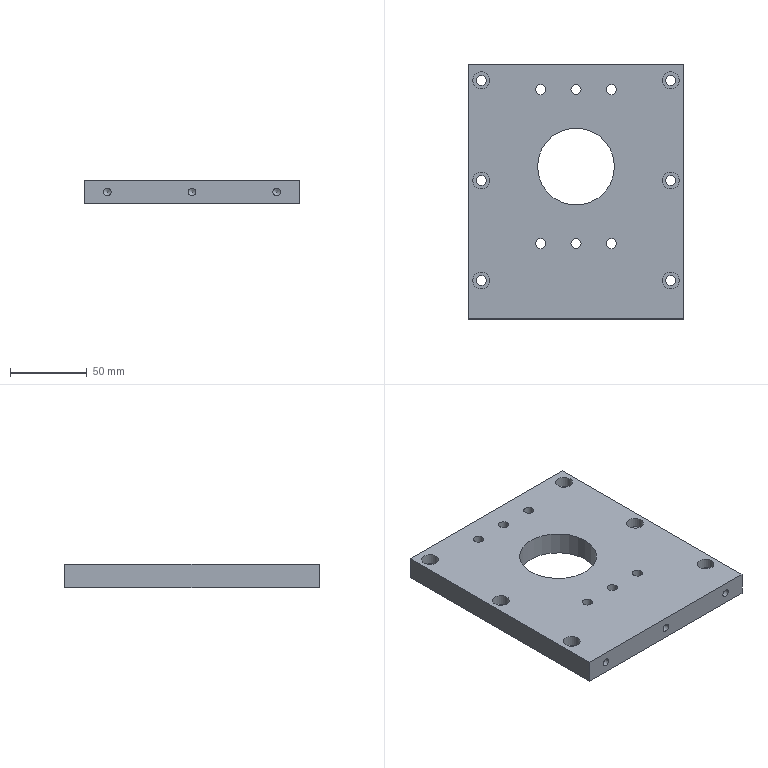Part | NX | 1 solid | 49 faces | box 140 x 165 x 15 mm | volume 305013 mm3 | cylinder 28 | plane 18 | cone 3 | commonest cylinder face diameters 6.6 x12 11 x12 5 x3 50 x1
STEP:
#1=CARTESIAN_POINT('',(-70.,82.5,7.5));
#2=VERTEX_POINT('',#1);
#3=CARTESIAN_POINT('',(-70.,82.5,-7.5));
#4=VERTEX_POINT('',#3);
#5=CARTESIAN_POINT('',(-70.,82.5,7.5));
#6=DIRECTION('',(0.,0.,-1.));
#7=VECTOR('',#6,1000.);
#8=LINE('',#5,#7);
#9=EDGE_CURVE('',#2,#4,#8,.T.);
#10=ORIENTED_EDGE('',*,*,#9,.F.);
#11=CARTESIAN_POINT('',(70.,82.5,7.5));
#12=VERTEX_POINT('',#11);
#13=CARTESIAN_POINT('',(-75.,82.5,7.5));
#14=DIRECTION('',(-1.,0.,0.));
#15=VECTOR('',#14,1000.);
#16=LINE('',#13,#15);
#17=EDGE_CURVE('',#12,#2,#16,.T.);
#18=ORIENTED_EDGE('',*,*,#17,.F.);
#19=CARTESIAN_POINT('',(70.,82.5,-7.5));
#20=VERTEX_POINT('',#19);
#21=CARTESIAN_POINT('',(70.,82.5,7.5));
#22=DIRECTION('',(0.,0.,-1.));
#23=VECTOR('',#22,1000.);
#24=LINE('',#21,#23);
#25=EDGE_CURVE('',#12,#20,#24,.T.);
#26=ORIENTED_EDGE('',*,*,#25,.T.);
#27=CARTESIAN_POINT('',(-75.,82.5,-7.5));
#28=DIRECTION('',(-1.,0.,0.));
#29=VECTOR('',#28,1000.);
#30=LINE('',#27,#29);
#31=EDGE_CURVE('',#20,#4,#30,.T.);
#32=ORIENTED_EDGE('',*,*,#31,.T.);
#33=EDGE_LOOP('',(#10,#18,#26,#32));
#34=FACE_BOUND('',#33,.T.);
#35=CARTESIAN_POINT('',(-75.,82.5,7.5));
#36=DIRECTION('',(0.,-1.,0.));
#37=DIRECTION('',(0.,0.,-1.));
#38=AXIS2_PLACEMENT_3D('',#35,#36,#37);
#39=PLANE('',#38);
#40=ADVANCED_FACE('',(#34),#39,.F.);
#41=CARTESIAN_POINT('',(0.,-82.5,-2.5));
#42=VERTEX_POINT('',#41);
#43=CARTESIAN_POINT('',(0.,-82.5,0.));
#44=DIRECTION('',(0.,-1.,0.));
#45=DIRECTION('',(0.,0.,-1.));
#46=AXIS2_PLACEMENT_3D('',#43,#44,#45);
#47=CIRCLE('',#46,2.5);
#48=EDGE_CURVE('',#42,#42,#47,.T.);
#49=ORIENTED_EDGE('',*,*,#48,.F.);
#50=EDGE_LOOP('',(#49));
#51=FACE_BOUND('',#50,.T.);
#52=CARTESIAN_POINT('',(55.,-82.5,-2.5));
#53=VERTEX_POINT('',#52);
#54=CARTESIAN_POINT('',(55.,-82.5,0.));
#55=DIRECTION('',(0.,-1.,0.));
#56=DIRECTION('',(0.,0.,-1.));
#57=AXIS2_PLACEMENT_3D('',#54,#55,#56);
#58=CIRCLE('',#57,2.5);
#59=EDGE_CURVE('',#53,#53,#58,.T.);
#60=ORIENTED_EDGE('',*,*,#59,.F.);
#61=EDGE_LOOP('',(#60));
#62=FACE_BOUND('',#61,.T.);
#63=CARTESIAN_POINT('',(-55.,-82.5,-2.5));
#64=VERTEX_POINT('',#63);
#65=CARTESIAN_POINT('',(-55.,-82.5,0.));
#66=DIRECTION('',(0.,-1.,0.));
#67=DIRECTION('',(0.,0.,-1.));
#68=AXIS2_PLACEMENT_3D('',#65,#66,#67);
#69=CIRCLE('',#68,2.5);
#70=EDGE_CURVE('',#64,#64,#69,.T.);
#71=ORIENTED_EDGE('',*,*,#70,.F.);
#72=EDGE_LOOP('',(#71));
#73=FACE_BOUND('',#72,.T.);
#74=CARTESIAN_POINT('',(-70.,-82.5,7.5));
#75=VERTEX_POINT('',#74);
#76=CARTESIAN_POINT('',(-70.,-82.5,-7.5));
#77=VERTEX_POINT('',#76);
#78=CARTESIAN_POINT('',(-70.,-82.5,7.5));
#79=DIRECTION('',(0.,0.,-1.));
#80=VECTOR('',#79,1000.);
#81=LINE('',#78,#80);
#82=EDGE_CURVE('',#75,#77,#81,.T.);
#83=ORIENTED_EDGE('',*,*,#82,.T.);
#84=CARTESIAN_POINT('',(70.,-82.5,-7.5));
#85=VERTEX_POINT('',#84);
#86=CARTESIAN_POINT('',(-75.,-82.5,-7.5));
#87=DIRECTION('',(1.,0.,0.));
#88=VECTOR('',#87,1000.);
#89=LINE('',#86,#88);
#90=EDGE_CURVE('',#77,#85,#89,.T.);
#91=ORIENTED_EDGE('',*,*,#90,.T.);
#92=CARTESIAN_POINT('',(70.,-82.5,7.5));
#93=VERTEX_POINT('',#92);
#94=CARTESIAN_POINT('',(70.,-82.5,7.5));
#95=DIRECTION('',(0.,0.,-1.));
#96=VECTOR('',#95,1000.);
#97=LINE('',#94,#96);
#98=EDGE_CURVE('',#93,#85,#97,.T.);
#99=ORIENTED_EDGE('',*,*,#98,.F.);
#100=CARTESIAN_POINT('',(-75.,-82.5,7.5));
#101=DIRECTION('',(1.,0.,0.));
#102=VECTOR('',#101,1000.);
#103=LINE('',#100,#102);
#104=EDGE_CURVE('',#75,#93,#103,.T.);
#105=ORIENTED_EDGE('',*,*,#104,.F.);
#106=EDGE_LOOP('',(#83,#91,#99,#105));
#107=FACE_BOUND('',#106,.T.);
#108=CARTESIAN_POINT('',(-75.,-82.5,7.5));
#109=DIRECTION('',(0.,1.,0.));
#110=DIRECTION('',(0.,0.,1.));
#111=AXIS2_PLACEMENT_3D('',#108,#109,#110);
#112=PLANE('',#111);
#113=ADVANCED_FACE('',(#51,#62,#73,#107),#112,.F.);
#114=CARTESIAN_POINT('',(-25.,16.5,7.5));
#115=VERTEX_POINT('',#114);
#116=CARTESIAN_POINT('',(0.,16.5,7.5));
#117=DIRECTION('',(0.,0.,-1.));
#118=DIRECTION('',(-1.,0.,0.));
#119=AXIS2_PLACEMENT_3D('',#116,#117,#118);
#120=CIRCLE('',#119,25.);
#121=EDGE_CURVE('',#115,#115,#120,.T.);
#122=ORIENTED_EDGE('',*,*,#121,.T.);
#123=EDGE_LOOP('',(#122));
#124=FACE_BOUND('',#123,.T.);
#125=CARTESIAN_POINT('',(19.7,66.5,7.5));
#126=VERTEX_POINT('',#125);
#127=CARTESIAN_POINT('',(23.,66.5,7.5));
#128=DIRECTION('',(0.,0.,-1.));
#129=DIRECTION('',(-1.,0.,0.));
#130=AXIS2_PLACEMENT_3D('',#127,#128,#129);
#131=CIRCLE('',#130,3.3);
#132=EDGE_CURVE('',#126,#126,#131,.T.);
#133=ORIENTED_EDGE('',*,*,#132,.T.);
#134=EDGE_LOOP('',(#133));
#135=FACE_BOUND('',#134,.T.);
#136=CARTESIAN_POINT('',(-26.3,66.5,7.5));
#137=VERTEX_POINT('',#136);
#138=CARTESIAN_POINT('',(-23.,66.5,7.5));
#139=DIRECTION('',(0.,0.,-1.));
#140=DIRECTION('',(-1.,0.,0.));
#141=AXIS2_PLACEMENT_3D('',#138,#139,#140);
#142=CIRCLE('',#141,3.3);
#143=EDGE_CURVE('',#137,#137,#142,.T.);
#144=ORIENTED_EDGE('',*,*,#143,.T.);
#145=EDGE_LOOP('',(#144));
#146=FACE_BOUND('',#145,.T.);
#147=CARTESIAN_POINT('',(-3.3,66.5,7.5));
#148=VERTEX_POINT('',#147);
#149=CARTESIAN_POINT('',(0.,66.5,7.5));
#150=DIRECTION('',(0.,0.,-1.));
#151=DIRECTION('',(-1.,0.,0.));
#152=AXIS2_PLACEMENT_3D('',#149,#150,#151);
#153=CIRCLE('',#152,3.3);
#154=EDGE_CURVE('',#148,#148,#153,.T.);
#155=ORIENTED_EDGE('',*,*,#154,.T.);
#156=EDGE_LOOP('',(#155));
#157=FACE_BOUND('',#156,.T.);
#158=CARTESIAN_POINT('',(-3.3,-33.5,7.5));
#159=VERTEX_POINT('',#158);
#160=CARTESIAN_POINT('',(0.,-33.5,7.5));
#161=DIRECTION('',(0.,0.,-1.));
#162=DIRECTION('',(-1.,0.,0.));
#163=AXIS2_PLACEMENT_3D('',#160,#161,#162);
#164=CIRCLE('',#163,3.3);
#165=EDGE_CURVE('',#159,#159,#164,.T.);
#166=ORIENTED_EDGE('',*,*,#165,.T.);
#167=EDGE_LOOP('',(#166));
#168=FACE_BOUND('',#167,.T.);
#169=CARTESIAN_POINT('',(19.7,-33.5,7.5));
#170=VERTEX_POINT('',#169);
#171=CARTESIAN_POINT('',(23.,-33.5,7.5));
#172=DIRECTION('',(0.,0.,-1.));
#173=DIRECTION('',(-1.,0.,0.));
#174=AXIS2_PLACEMENT_3D('',#171,#172,#173);
#175=CIRCLE('',#174,3.3);
#176=EDGE_CURVE('',#170,#170,#175,.T.);
#177=ORIENTED_EDGE('',*,*,#176,.T.);
#178=EDGE_LOOP('',(#177));
#179=FACE_BOUND('',#178,.T.);
#180=CARTESIAN_POINT('',(-26.3,-33.5,7.5));
#181=VERTEX_POINT('',#180);
#182=CARTESIAN_POINT('',(-23.,-33.5,7.5));
#183=DIRECTION('',(0.,0.,-1.));
#184=DIRECTION('',(-1.,0.,0.));
#185=AXIS2_PLACEMENT_3D('',#182,#183,#184);
#186=CIRCLE('',#185,3.3);
#187=EDGE_CURVE('',#181,#181,#186,.T.);
#188=ORIENTED_EDGE('',*,*,#187,.T.);
#189=EDGE_LOOP('',(#188));
#190=FACE_BOUND('',#189,.T.);
#191=CARTESIAN_POINT('',(-56.,-57.5,7.5));
#192=VERTEX_POINT('',#191);
#193=CARTESIAN_POINT('',(-61.5,-57.5,7.5));
#194=DIRECTION('',(0.,0.,1.));
#195=DIRECTION('',(1.,0.,0.));
#196=AXIS2_PLACEMENT_3D('',#193,#194,#195);
#197=CIRCLE('',#196,5.5);
#198=EDGE_CURVE('',#192,#192,#197,.T.);
#199=ORIENTED_EDGE('',*,*,#198,.F.);
#200=EDGE_LOOP('',(#199));
#201=FACE_BOUND('',#200,.T.);
#202=CARTESIAN_POINT('',(-56.,7.5,7.5));
#203=VERTEX_POINT('',#202);
#204=CARTESIAN_POINT('',(-61.5,7.5,7.5));
#205=DIRECTION('',(0.,0.,1.));
#206=DIRECTION('',(1.,0.,0.));
#207=AXIS2_PLACEMENT_3D('',#204,#205,#206);
#208=CIRCLE('',#207,5.5);
#209=EDGE_CURVE('',#203,#203,#208,.T.);
#210=ORIENTED_EDGE('',*,*,#209,.F.);
#211=EDGE_LOOP('',(#210));
#212=FACE_BOUND('',#211,.T.);
#213=CARTESIAN_POINT('',(-56.,72.5,7.5));
#214=VERTEX_POINT('',#213);
#215=CARTESIAN_POINT('',(-61.5,72.5,7.5));
#216=DIRECTION('',(0.,0.,1.));
#217=DIRECTION('',(1.,0.,0.));
#218=AXIS2_PLACEMENT_3D('',#215,#216,#217);
#219=CIRCLE('',#218,5.5);
#220=EDGE_CURVE('',#214,#214,#219,.T.);
#221=ORIENTED_EDGE('',*,*,#220,.F.);
#222=EDGE_LOOP('',(#221));
#223=FACE_BOUND('',#222,.T.);
#224=CARTESIAN_POINT('',(67.,-57.5,7.5));
#225=VERTEX_POINT('',#224);
#226=CARTESIAN_POINT('',(61.5,-57.5,7.5));
#227=DIRECTION('',(0.,0.,1.));
#228=DIRECTION('',(1.,0.,0.));
#229=AXIS2_PLACEMENT_3D('',#226,#227,#228);
#230=CIRCLE('',#229,5.5);
#231=EDGE_CURVE('',#225,#225,#230,.T.);
#232=ORIENTED_EDGE('',*,*,#231,.F.);
#233=EDGE_LOOP('',(#232));
#234=FACE_BOUND('',#233,.T.);
#235=CARTESIAN_POINT('',(67.,7.5,7.5));
#236=VERTEX_POINT('',#235);
#237=CARTESIAN_POINT('',(61.5,7.5,7.5));
#238=DIRECTION('',(0.,0.,1.));
#239=DIRECTION('',(1.,0.,0.));
#240=AXIS2_PLACEMENT_3D('',#237,#238,#239);
#241=CIRCLE('',#240,5.5);
#242=EDGE_CURVE('',#236,#236,#241,.T.);
#243=ORIENTED_EDGE('',*,*,#242,.F.);
#244=EDGE_LOOP('',(#243));
#245=FACE_BOUND('',#244,.T.);
#246=CARTESIAN_POINT('',(67.,72.5,7.5));
#247=VERTEX_POINT('',#246);
#248=CARTESIAN_POINT('',(61.5,72.5,7.5));
#249=DIRECTION('',(0.,0.,1.));
#250=DIRECTION('',(1.,0.,0.));
#251=AXIS2_PLACEMENT_3D('',#248,#249,#250);
#252=CIRCLE('',#251,5.5);
#253=EDGE_CURVE('',#247,#247,#252,.T.);
#254=ORIENTED_EDGE('',*,*,#253,.F.);
#255=EDGE_LOOP('',(#254));
#256=FACE_BOUND('',#255,.T.);
#257=ORIENTED_EDGE('',*,*,#17,.T.);
#258=CARTESIAN_POINT('',(-70.,82.5,7.5));
#259=DIRECTION('',(0.,1.,0.));
#260=VECTOR('',#259,1000.);
#261=LINE('',#258,#260);
#262=EDGE_CURVE('',#75,#2,#261,.T.);
#263=ORIENTED_EDGE('',*,*,#262,.F.);
#264=ORIENTED_EDGE('',*,*,#104,.T.);
#265=CARTESIAN_POINT('',(70.,82.5,7.5));
#266=DIRECTION('',(0.,1.,0.));
#267=VECTOR('',#266,1000.);
#268=LINE('',#265,#267);
#269=EDGE_CURVE('',#93,#12,#268,.T.);
#270=ORIENTED_EDGE('',*,*,#269,.T.);
#271=EDGE_LOOP('',(#257,#263,#264,#270));
#272=FACE_BOUND('',#271,.T.);
#273=CARTESIAN_POINT('',(0.,0.,7.5));
#274=DIRECTION('',(0.,0.,1.));
#275=DIRECTION('',(1.,0.,0.));
#276=AXIS2_PLACEMENT_3D('',#273,#274,#275);
#277=PLANE('',#276);
#278=ADVANCED_FACE('',(#124,#135,#146,#157,#168,#179,#190,#201,#212,#223,#234,#245,#256,#272),#277,.T.);
#279=CARTESIAN_POINT('',(-25.,16.5,-7.5));
#280=VERTEX_POINT('',#279);
#281=CARTESIAN_POINT('',(0.,16.5,-7.5));
#282=DIRECTION('',(0.,0.,-1.));
#283=DIRECTION('',(-1.,0.,0.));
#284=AXIS2_PLACEMENT_3D('',#281,#282,#283);
#285=CIRCLE('',#284,25.);
#286=EDGE_CURVE('',#280,#280,#285,.T.);
#287=ORIENTED_EDGE('',*,*,#286,.F.);
#288=EDGE_LOOP('',(#287));
#289=FACE_BOUND('',#288,.T.);
#290=CARTESIAN_POINT('',(17.5,66.5,-7.5));
#291=VERTEX_POINT('',#290);
#292=CARTESIAN_POINT('',(23.,66.5,-7.5));
#293=DIRECTION('',(0.,0.,-1.));
#294=DIRECTION('',(-1.,0.,0.));
#295=AXIS2_PLACEMENT_3D('',#292,#293,#294);
#296=CIRCLE('',#295,5.5);
#297=EDGE_CURVE('',#291,#291,#296,.T.);
#298=ORIENTED_EDGE('',*,*,#297,.F.);
#299=EDGE_LOOP('',(#298));
#300=FACE_BOUND('',#299,.T.);
#301=CARTESIAN_POINT('',(-28.5,66.5,-7.5));
#302=VERTEX_POINT('',#301);
#303=CARTESIAN_POINT('',(-23.,66.5,-7.5));
#304=DIRECTION('',(0.,0.,-1.));
#305=DIRECTION('',(-1.,0.,0.));
#306=AXIS2_PLACEMENT_3D('',#303,#304,#305);
#307=CIRCLE('',#306,5.5);
#308=EDGE_CURVE('',#302,#302,#307,.T.);
#309=ORIENTED_EDGE('',*,*,#308,.F.);
#310=EDGE_LOOP('',(#309));
#311=FACE_BOUND('',#310,.T.);
#312=CARTESIAN_POINT('',(-5.5,66.5,-7.5));
#313=VERTEX_POINT('',#312);
#314=CARTESIAN_POINT('',(0.,66.5,-7.5));
#315=DIRECTION('',(0.,0.,-1.));
#316=DIRECTION('',(-1.,0.,0.));
#317=AXIS2_PLACEMENT_3D('',#314,#315,#316);
#318=CIRCLE('',#317,5.5);
#319=EDGE_CURVE('',#313,#313,#318,.T.);
#320=ORIENTED_EDGE('',*,*,#319,.F.);
#321=EDGE_LOOP('',(#320));
#322=FACE_BOUND('',#321,.T.);
#323=CARTESIAN_POINT('',(-5.5,-33.5,-7.5));
#324=VERTEX_POINT('',#323);
#325=CARTESIAN_POINT('',(0.,-33.5,-7.5));
#326=DIRECTION('',(0.,0.,-1.));
#327=DIRECTION('',(-1.,0.,0.));
#328=AXIS2_PLACEMENT_3D('',#325,#326,#327);
#329=CIRCLE('',#328,5.5);
#330=EDGE_CURVE('',#324,#324,#329,.T.);
#331=ORIENTED_EDGE('',*,*,#330,.F.);
#332=EDGE_LOOP('',(#331));
#333=FACE_BOUND('',#332,.T.);
#334=CARTESIAN_POINT('',(17.5,-33.5,-7.5));
#335=VERTEX_POINT('',#334);
#336=CARTESIAN_POINT('',(23.,-33.5,-7.5));
#337=DIRECTION('',(0.,0.,-1.));
#338=DIRECTION('',(-1.,0.,0.));
#339=AXIS2_PLACEMENT_3D('',#336,#337,#338);
#340=CIRCLE('',#339,5.5);
#341=EDGE_CURVE('',#335,#335,#340,.T.);
#342=ORIENTED_EDGE('',*,*,#341,.F.);
#343=EDGE_LOOP('',(#342));
#344=FACE_BOUND('',#343,.T.);
#345=CARTESIAN_POINT('',(-28.5,-33.5,-7.5));
#346=VERTEX_POINT('',#345);
#347=CARTESIAN_POINT('',(-23.,-33.5,-7.5));
#348=DIRECTION('',(0.,0.,-1.));
#349=DIRECTION('',(-1.,0.,0.));
#350=AXIS2_PLACEMENT_3D('',#347,#348,#349);
#351=CIRCLE('',#350,5.5);
#352=EDGE_CURVE('',#346,#346,#351,.T.);
#353=ORIENTED_EDGE('',*,*,#352,.F.);
#354=EDGE_LOOP('',(#353));
#355=FACE_BOUND('',#354,.T.);
#356=CARTESIAN_POINT('',(-58.2,-57.5,-7.5));
#357=VERTEX_POINT('',#356);
#358=CARTESIAN_POINT('',(-61.5,-57.5,-7.5));
#359=DIRECTION('',(0.,0.,1.));
#360=DIRECTION('',(1.,0.,0.));
#361=AXIS2_PLACEMENT_3D('',#358,#359,#360);
#362=CIRCLE('',#361,3.3);
#363=EDGE_CURVE('',#357,#357,#362,.T.);
#364=ORIENTED_EDGE('',*,*,#363,.T.);
#365=EDGE_LOOP('',(#364));
#366=FACE_BOUND('',#365,.T.);
#367=CARTESIAN_POINT('',(-58.2,7.5,-7.5));
#368=VERTEX_POINT('',#367);
#369=CARTESIAN_POINT('',(-61.5,7.5,-7.5));
#370=DIRECTION('',(0.,0.,1.));
#371=DIRECTION('',(1.,0.,0.));
#372=AXIS2_PLACEMENT_3D('',#369,#370,#371);
#373=CIRCLE('',#372,3.3);
#374=EDGE_CURVE('',#368,#368,#373,.T.);
#375=ORIENTED_EDGE('',*,*,#374,.T.);
#376=EDGE_LOOP('',(#375));
#377=FACE_BOUND('',#376,.T.);
#378=CARTESIAN_POINT('',(-58.2,72.5,-7.5));
#379=VERTEX_POINT('',#378);
#380=CARTESIAN_POINT('',(-61.5,72.5,-7.5));
#381=DIRECTION('',(0.,0.,1.));
#382=DIRECTION('',(1.,0.,0.));
#383=AXIS2_PLACEMENT_3D('',#380,#381,#382);
#384=CIRCLE('',#383,3.3);
#385=EDGE_CURVE('',#379,#379,#384,.T.);
#386=ORIENTED_EDGE('',*,*,#385,.T.);
#387=EDGE_LOOP('',(#386));
#388=FACE_BOUND('',#387,.T.);
#389=CARTESIAN_POINT('',(64.8,-57.5,-7.5));
#390=VERTEX_POINT('',#389);
#391=CARTESIAN_POINT('',(61.5,-57.5,-7.5));
#392=DIRECTION('',(0.,0.,1.));
#393=DIRECTION('',(1.,0.,0.));
#394=AXIS2_PLACEMENT_3D('',#391,#392,#393);
#395=CIRCLE('',#394,3.3);
#396=EDGE_CURVE('',#390,#390,#395,.T.);
#397=ORIENTED_EDGE('',*,*,#396,.T.);
#398=EDGE_LOOP('',(#397));
#399=FACE_BOUND('',#398,.T.);
#400=CARTESIAN_POINT('',(64.8,7.5,-7.5));
#401=VERTEX_POINT('',#400);
#402=CARTESIAN_POINT('',(61.5,7.5,-7.5));
#403=DIRECTION('',(0.,0.,1.));
#404=DIRECTION('',(1.,0.,0.));
#405=AXIS2_PLACEMENT_3D('',#402,#403,#404);
#406=CIRCLE('',#405,3.3);
#407=EDGE_CURVE('',#401,#401,#406,.T.);
#408=ORIENTED_EDGE('',*,*,#407,.T.);
#409=EDGE_LOOP('',(#408));
#410=FACE_BOUND('',#409,.T.);
#411=CARTESIAN_POINT('',(64.8,72.5,-7.5));
#412=VERTEX_POINT('',#411);
#413=CARTESIAN_POINT('',(61.5,72.5,-7.5));
#414=DIRECTION('',(0.,0.,1.));
#415=DIRECTION('',(1.,0.,0.));
#416=AXIS2_PLACEMENT_3D('',#413,#414,#415);
#417=CIRCLE('',#416,3.3);
#418=EDGE_CURVE('',#412,#412,#417,.T.);
#419=ORIENTED_EDGE('',*,*,#418,.T.);
#420=EDGE_LOOP('',(#419));
#421=FACE_BOUND('',#420,.T.);
#422=CARTESIAN_POINT('',(-70.,82.5,-7.5));
#423=DIRECTION('',(0.,1.,0.));
#424=VECTOR('',#423,1000.);
#425=LINE('',#422,#424);
#426=EDGE_CURVE('',#77,#4,#425,.T.);
#427=ORIENTED_EDGE('',*,*,#426,.T.);
#428=ORIENTED_EDGE('',*,*,#31,.F.);
#429=CARTESIAN_POINT('',(70.,82.5,-7.5));
#430=DIRECTION('',(0.,1.,0.));
#431=VECTOR('',#430,1000.);
#432=LINE('',#429,#431);
#433=EDGE_CURVE('',#85,#20,#432,.T.);
#434=ORIENTED_EDGE('',*,*,#433,.F.);
#435=ORIENTED_EDGE('',*,*,#90,.F.);
#436=EDGE_LOOP('',(#427,#428,#434,#435));
#437=FACE_BOUND('',#436,.T.);
#438=CARTESIAN_POINT('',(0.,0.,-7.5));
#439=DIRECTION('',(0.,0.,1.));
#440=DIRECTION('',(1.,0.,0.));
#441=AXIS2_PLACEMENT_3D('',#438,#439,#440);
#442=PLANE('',#441);
#443=ADVANCED_FACE('',(#289,#300,#311,#322,#333,#344,#355,#366,#377,#388,#399,#410,#421,#437),#442,.F.);
#444=ORIENTED_EDGE('',*,*,#132,.F.);
#445=EDGE_LOOP('',(#444));
#446=FACE_BOUND('',#445,.T.);
#447=CARTESIAN_POINT('',(19.7,66.5,-0.7));
#448=VERTEX_POINT('',#447);
#449=CARTESIAN_POINT('',(23.,66.5,-0.7));
#450=DIRECTION('',(0.,0.,-1.));
#451=DIRECTION('',(-1.,0.,0.));
#452=AXIS2_PLACEMENT_3D('',#449,#450,#451);
#453=CIRCLE('',#452,3.3);
#454=EDGE_CURVE('',#448,#448,#453,.T.);
#455=ORIENTED_EDGE('',*,*,#454,.T.);
#456=EDGE_LOOP('',(#455));
#457=FACE_BOUND('',#456,.T.);
#458=CARTESIAN_POINT('',(23.,66.5,-7.5));
#459=DIRECTION('',(0.,0.,-1.));
#460=DIRECTION('',(-1.,0.,0.));
#461=AXIS2_PLACEMENT_3D('',#458,#459,#460);
#462=CYLINDRICAL_SURFACE('',#461,3.3);
#463=ADVANCED_FACE('',(#446,#457),#462,.F.);
#464=ORIENTED_EDGE('',*,*,#454,.F.);
#465=EDGE_LOOP('',(#464));
#466=FACE_BOUND('',#465,.T.);
#467=CARTESIAN_POINT('',(17.5,66.5,-0.7));
#468=VERTEX_POINT('',#467);
#469=CARTESIAN_POINT('',(23.,66.5,-0.7));
#470=DIRECTION('',(0.,0.,-1.));
#471=DIRECTION('',(-1.,0.,0.));
#472=AXIS2_PLACEMENT_3D('',#469,#470,#471);
#473=CIRCLE('',#472,5.5);
#474=EDGE_CURVE('',#468,#468,#473,.T.);
#475=ORIENTED_EDGE('',*,*,#474,.T.);
#476=EDGE_LOOP('',(#475));
#477=FACE_BOUND('',#476,.T.);
#478=CARTESIAN_POINT('',(26.3,66.5,-0.7));
#479=DIRECTION('',(0.,0.,1.));
#480=DIRECTION('',(1.,0.,0.));
#481=AXIS2_PLACEMENT_3D('',#478,#479,#480);
#482=PLANE('',#481);
#483=ADVANCED_FACE('',(#466,#477),#482,.F.);
#484=ORIENTED_EDGE('',*,*,#474,.F.);
#485=EDGE_LOOP('',(#484));
#486=FACE_BOUND('',#485,.T.);
#487=ORIENTED_EDGE('',*,*,#297,.T.);
#488=EDGE_LOOP('',(#487));
#489=FACE_BOUND('',#488,.T.);
#490=CARTESIAN_POINT('',(23.,66.5,-7.5));
#491=DIRECTION('',(0.,0.,-1.));
#492=DIRECTION('',(-1.,0.,0.));
#493=AXIS2_PLACEMENT_3D('',#490,#491,#492);
#494=CYLINDRICAL_SURFACE('',#493,5.5);
#495=ADVANCED_FACE('',(#486,#489),#494,.F.);
#496=ORIENTED_EDGE('',*,*,#143,.F.);
#497=EDGE_LOOP('',(#496));
#498=FACE_BOUND('',#497,.T.);
#499=CARTESIAN_POINT('',(-26.3,66.5,-0.7));
#500=VERTEX_POINT('',#499);
#501=CARTESIAN_POINT('',(-23.,66.5,-0.7));
#502=DIRECTION('',(0.,0.,-1.));
#503=DIRECTION('',(-1.,0.,0.));
#504=AXIS2_PLACEMENT_3D('',#501,#502,#503);
#505=CIRCLE('',#504,3.3);
#506=EDGE_CURVE('',#500,#500,#505,.T.);
#507=ORIENTED_EDGE('',*,*,#506,.T.);
#508=EDGE_LOOP('',(#507));
#509=FACE_BOUND('',#508,.T.);
#510=CARTESIAN_POINT('',(-23.,66.5,-7.5));
#511=DIRECTION('',(0.,0.,-1.));
#512=DIRECTION('',(-1.,0.,0.));
#513=AXIS2_PLACEMENT_3D('',#510,#511,#512);
#514=CYLINDRICAL_SURFACE('',#513,3.3);
#515=ADVANCED_FACE('',(#498,#509),#514,.F.);
#516=ORIENTED_EDGE('',*,*,#506,.F.);
#517=EDGE_LOOP('',(#516));
#518=FACE_BOUND('',#517,.T.);
#519=CARTESIAN_POINT('',(-28.5,66.5,-0.7));
#520=VERTEX_POINT('',#519);
#521=CARTESIAN_POINT('',(-23.,66.5,-0.7));
#522=DIRECTION('',(0.,0.,-1.));
#523=DIRECTION('',(-1.,0.,0.));
#524=AXIS2_PLACEMENT_3D('',#521,#522,#523);
#525=CIRCLE('',#524,5.5);
#526=EDGE_CURVE('',#520,#520,#525,.T.);
#527=ORIENTED_EDGE('',*,*,#526,.T.);
#528=EDGE_LOOP('',(#527));
#529=FACE_BOUND('',#528,.T.);
#530=CARTESIAN_POINT('',(-19.7,66.5,-0.7));
#531=DIRECTION('',(0.,0.,1.));
#532=DIRECTION('',(1.,0.,0.));
#533=AXIS2_PLACEMENT_3D('',#530,#531,#532);
#534=PLANE('',#533);
#535=ADVANCED_FACE('',(#518,#529),#534,.F.);
#536=ORIENTED_EDGE('',*,*,#526,.F.);
#537=EDGE_LOOP('',(#536));
#538=FACE_BOUND('',#537,.T.);
#539=ORIENTED_EDGE('',*,*,#308,.T.);
#540=EDGE_LOOP('',(#539));
#541=FACE_BOUND('',#540,.T.);
#542=CARTESIAN_POINT('',(-23.,66.5,-7.5));
#543=DIRECTION('',(0.,0.,-1.));
#544=DIRECTION('',(-1.,0.,0.));
#545=AXIS2_PLACEMENT_3D('',#542,#543,#544);
#546=CYLINDRICAL_SURFACE('',#545,5.5);
#547=ADVANCED_FACE('',(#538,#541),#546,.F.);
#548=ORIENTED_EDGE('',*,*,#154,.F.);
#549=EDGE_LOOP('',(#548));
#550=FACE_BOUND('',#549,.T.);
#551=CARTESIAN_POINT('',(-3.3,66.5,-0.7));
#552=VERTEX_POINT('',#551);
#553=CARTESIAN_POINT('',(0.,66.5,-0.7));
#554=DIRECTION('',(0.,0.,-1.));
#555=DIRECTION('',(-1.,0.,0.));
#556=AXIS2_PLACEMENT_3D('',#553,#554,#555);
#557=CIRCLE('',#556,3.3);
#558=EDGE_CURVE('',#552,#552,#557,.T.);
#559=ORIENTED_EDGE('',*,*,#558,.T.);
#560=EDGE_LOOP('',(#559));
#561=FACE_BOUND('',#560,.T.);
#562=CARTESIAN_POINT('',(0.,66.5,-7.5));
#563=DIRECTION('',(0.,0.,-1.));
#564=DIRECTION('',(-1.,0.,0.));
#565=AXIS2_PLACEMENT_3D('',#562,#563,#564);
#566=CYLINDRICAL_SURFACE('',#565,3.3);
#567=ADVANCED_FACE('',(#550,#561),#566,.F.);
#568=ORIENTED_EDGE('',*,*,#558,.F.);
#569=EDGE_LOOP('',(#568));
#570=FACE_BOUND('',#569,.T.);
#571=CARTESIAN_POINT('',(-5.5,66.5,-0.7));
#572=VERTEX_POINT('',#571);
#573=CARTESIAN_POINT('',(0.,66.5,-0.7));
#574=DIRECTION('',(0.,0.,-1.));
#575=DIRECTION('',(-1.,0.,0.));
#576=AXIS2_PLACEMENT_3D('',#573,#574,#575);
#577=CIRCLE('',#576,5.5);
#578=EDGE_CURVE('',#572,#572,#577,.T.);
#579=ORIENTED_EDGE('',*,*,#578,.T.);
#580=EDGE_LOOP('',(#579));
#581=FACE_BOUND('',#580,.T.);
#582=CARTESIAN_POINT('',(3.3,66.5,-0.7));
#583=DIRECTION('',(0.,0.,1.));
#584=DIRECTION('',(1.,0.,0.));
#585=AXIS2_PLACEMENT_3D('',#582,#583,#584);
#586=PLANE('',#585);
#587=ADVANCED_FACE('',(#570,#581),#586,.F.);
#588=ORIENTED_EDGE('',*,*,#578,.F.);
#589=EDGE_LOOP('',(#588));
#590=FACE_BOUND('',#589,.T.);
#591=ORIENTED_EDGE('',*,*,#319,.T.);
#592=EDGE_LOOP('',(#591));
#593=FACE_BOUND('',#592,.T.);
#594=CARTESIAN_POINT('',(0.,66.5,-7.5));
#595=DIRECTION('',(0.,0.,-1.));
#596=DIRECTION('',(-1.,0.,0.));
#597=AXIS2_PLACEMENT_3D('',#594,#595,#596);
#598=CYLINDRICAL_SURFACE('',#597,5.5);
#599=ADVANCED_FACE('',(#590,#593),#598,.F.);
#600=ORIENTED_EDGE('',*,*,#165,.F.);
#601=EDGE_LOOP('',(#600));
#602=FACE_BOUND('',#601,.T.);
#603=CARTESIAN_POINT('',(-3.3,-33.5,-0.7));
#604=VERTEX_POINT('',#603);
#605=CARTESIAN_POINT('',(0.,-33.5,-0.7));
#606=DIRECTION('',(0.,0.,-1.));
#607=DIRECTION('',(-1.,0.,0.));
#608=AXIS2_PLACEMENT_3D('',#605,#606,#607);
#609=CIRCLE('',#608,3.3);
#610=EDGE_CURVE('',#604,#604,#609,.T.);
#611=ORIENTED_EDGE('',*,*,#610,.T.);
#612=EDGE_LOOP('',(#611));
#613=FACE_BOUND('',#612,.T.);
#614=CARTESIAN_POINT('',(0.,-33.5,-7.5));
#615=DIRECTION('',(0.,0.,-1.));
#616=DIRECTION('',(-1.,0.,0.));
#617=AXIS2_PLACEMENT_3D('',#614,#615,#616);
#618=CYLINDRICAL_SURFACE('',#617,3.3);
#619=ADVANCED_FACE('',(#602,#613),#618,.F.);
#620=ORIENTED_EDGE('',*,*,#610,.F.);
#621=EDGE_LOOP('',(#620));
#622=FACE_BOUND('',#621,.T.);
#623=CARTESIAN_POINT('',(-5.5,-33.5,-0.7));
#624=VERTEX_POINT('',#623);
#625=CARTESIAN_POINT('',(0.,-33.5,-0.7));
#626=DIRECTION('',(0.,0.,-1.));
#627=DIRECTION('',(-1.,0.,0.));
#628=AXIS2_PLACEMENT_3D('',#625,#626,#627);
#629=CIRCLE('',#628,5.5);
#630=EDGE_CURVE('',#624,#624,#629,.T.);
#631=ORIENTED_EDGE('',*,*,#630,.T.);
#632=EDGE_LOOP('',(#631));
#633=FACE_BOUND('',#632,.T.);
#634=CARTESIAN_POINT('',(3.3,-33.5,-0.7));
#635=DIRECTION('',(0.,0.,1.));
#636=DIRECTION('',(1.,0.,0.));
#637=AXIS2_PLACEMENT_3D('',#634,#635,#636);
#638=PLANE('',#637);
#639=ADVANCED_FACE('',(#622,#633),#638,.F.);
#640=ORIENTED_EDGE('',*,*,#630,.F.);
#641=EDGE_LOOP('',(#640));
#642=FACE_BOUND('',#641,.T.);
#643=ORIENTED_EDGE('',*,*,#330,.T.);
#644=EDGE_LOOP('',(#643));
#645=FACE_BOUND('',#644,.T.);
#646=CARTESIAN_POINT('',(0.,-33.5,-7.5));
#647=DIRECTION('',(0.,0.,-1.));
#648=DIRECTION('',(-1.,0.,0.));
#649=AXIS2_PLACEMENT_3D('',#646,#647,#648);
#650=CYLINDRICAL_SURFACE('',#649,5.5);
#651=ADVANCED_FACE('',(#642,#645),#650,.F.);
#652=ORIENTED_EDGE('',*,*,#176,.F.);
#653=EDGE_LOOP('',(#652));
#654=FACE_BOUND('',#653,.T.);
#655=CARTESIAN_POINT('',(19.7,-33.5,-0.7));
#656=VERTEX_POINT('',#655);
#657=CARTESIAN_POINT('',(23.,-33.5,-0.7));
#658=DIRECTION('',(0.,0.,-1.));
#659=DIRECTION('',(-1.,0.,0.));
#660=AXIS2_PLACEMENT_3D('',#657,#658,#659);
#661=CIRCLE('',#660,3.3);
#662=EDGE_CURVE('',#656,#656,#661,.T.);
#663=ORIENTED_EDGE('',*,*,#662,.T.);
#664=EDGE_LOOP('',(#663));
#665=FACE_BOUND('',#664,.T.);
#666=CARTESIAN_POINT('',(23.,-33.5,-7.5));
#667=DIRECTION('',(0.,0.,-1.));
#668=DIRECTION('',(-1.,0.,0.));
#669=AXIS2_PLACEMENT_3D('',#666,#667,#668);
#670=CYLINDRICAL_SURFACE('',#669,3.3);
#671=ADVANCED_FACE('',(#654,#665),#670,.F.);
#672=ORIENTED_EDGE('',*,*,#662,.F.);
#673=EDGE_LOOP('',(#672));
#674=FACE_BOUND('',#673,.T.);
#675=CARTESIAN_POINT('',(17.5,-33.5,-0.7));
#676=VERTEX_POINT('',#675);
#677=CARTESIAN_POINT('',(23.,-33.5,-0.7));
#678=DIRECTION('',(0.,0.,-1.));
#679=DIRECTION('',(-1.,0.,0.));
#680=AXIS2_PLACEMENT_3D('',#677,#678,#679);
#681=CIRCLE('',#680,5.5);
#682=EDGE_CURVE('',#676,#676,#681,.T.);
#683=ORIENTED_EDGE('',*,*,#682,.T.);
#684=EDGE_LOOP('',(#683));
#685=FACE_BOUND('',#684,.T.);
#686=CARTESIAN_POINT('',(26.3,-33.5,-0.7));
#687=DIRECTION('',(0.,0.,1.));
#688=DIRECTION('',(1.,0.,0.));
#689=AXIS2_PLACEMENT_3D('',#686,#687,#688);
#690=PLANE('',#689);
#691=ADVANCED_FACE('',(#674,#685),#690,.F.);
#692=ORIENTED_EDGE('',*,*,#682,.F.);
#693=EDGE_LOOP('',(#692));
#694=FACE_BOUND('',#693,.T.);
#695=ORIENTED_EDGE('',*,*,#341,.T.);
#696=EDGE_LOOP('',(#695));
#697=FACE_BOUND('',#696,.T.);
#698=CARTESIAN_POINT('',(23.,-33.5,-7.5));
#699=DIRECTION('',(0.,0.,-1.));
#700=DIRECTION('',(-1.,0.,0.));
#701=AXIS2_PLACEMENT_3D('',#698,#699,#700);
#702=CYLINDRICAL_SURFACE('',#701,5.5);
#703=ADVANCED_FACE('',(#694,#697),#702,.F.);
#704=ORIENTED_EDGE('',*,*,#187,.F.);
#705=EDGE_LOOP('',(#704));
#706=FACE_BOUND('',#705,.T.);
#707=CARTESIAN_POINT('',(-26.3,-33.5,-0.7));
#708=VERTEX_POINT('',#707);
#709=CARTESIAN_POINT('',(-23.,-33.5,-0.7));
#710=DIRECTION('',(0.,0.,-1.));
#711=DIRECTION('',(-1.,0.,0.));
#712=AXIS2_PLACEMENT_3D('',#709,#710,#711);
#713=CIRCLE('',#712,3.3);
#714=EDGE_CURVE('',#708,#708,#713,.T.);
#715=ORIENTED_EDGE('',*,*,#714,.T.);
#716=EDGE_LOOP('',(#715));
#717=FACE_BOUND('',#716,.T.);
#718=CARTESIAN_POINT('',(-23.,-33.5,-7.5));
#719=DIRECTION('',(0.,0.,-1.));
#720=DIRECTION('',(-1.,0.,0.));
#721=AXIS2_PLACEMENT_3D('',#718,#719,#720);
#722=CYLINDRICAL_SURFACE('',#721,3.3);
#723=ADVANCED_FACE('',(#706,#717),#722,.F.);
#724=ORIENTED_EDGE('',*,*,#714,.F.);
#725=EDGE_LOOP('',(#724));
#726=FACE_BOUND('',#725,.T.);
#727=CARTESIAN_POINT('',(-28.5,-33.5,-0.7));
#728=VERTEX_POINT('',#727);
#729=CARTESIAN_POINT('',(-23.,-33.5,-0.7));
#730=DIRECTION('',(0.,0.,-1.));
#731=DIRECTION('',(-1.,0.,0.));
#732=AXIS2_PLACEMENT_3D('',#729,#730,#731);
#733=CIRCLE('',#732,5.5);
#734=EDGE_CURVE('',#728,#728,#733,.T.);
#735=ORIENTED_EDGE('',*,*,#734,.T.);
#736=EDGE_LOOP('',(#735));
#737=FACE_BOUND('',#736,.T.);
#738=CARTESIAN_POINT('',(-19.7,-33.5,-0.7));
#739=DIRECTION('',(0.,0.,1.));
#740=DIRECTION('',(1.,0.,0.));
#741=AXIS2_PLACEMENT_3D('',#738,#739,#740);
#742=PLANE('',#741);
#743=ADVANCED_FACE('',(#726,#737),#742,.F.);
#744=ORIENTED_EDGE('',*,*,#734,.F.);
#745=EDGE_LOOP('',(#744));
#746=FACE_BOUND('',#745,.T.);
#747=ORIENTED_EDGE('',*,*,#352,.T.);
#748=EDGE_LOOP('',(#747));
#749=FACE_BOUND('',#748,.T.);
#750=CARTESIAN_POINT('',(-23.,-33.5,-7.5));
#751=DIRECTION('',(0.,0.,-1.));
#752=DIRECTION('',(-1.,0.,0.));
#753=AXIS2_PLACEMENT_3D('',#750,#751,#752);
#754=CYLINDRICAL_SURFACE('',#753,5.5);
#755=ADVANCED_FACE('',(#746,#749),#754,.F.);
#756=CARTESIAN_POINT('',(0.,-65.998,0.));
#757=VERTEX_POINT('',#756);
#758=VERTEX_LOOP('',#757);
#759=FACE_BOUND('',#758,.T.);
#760=CARTESIAN_POINT('',(0.,-67.5,-2.5));
#761=VERTEX_POINT('',#760);
#762=CARTESIAN_POINT('',(0.,-67.5,0.));
#763=DIRECTION('',(0.,-1.,0.));
#764=DIRECTION('',(0.,0.,-1.));
#765=AXIS2_PLACEMENT_3D('',#762,#763,#764);
#766=CIRCLE('',#765,2.5);
#767=EDGE_CURVE('',#761,#761,#766,.T.);
#768=ORIENTED_EDGE('',*,*,#767,.T.);
#769=EDGE_LOOP('',(#768));
#770=FACE_BOUND('',#769,.T.);
#771=CARTESIAN_POINT('',(0.,-67.5,0.));
#772=DIRECTION('',(0.,-1.,0.));
#773=DIRECTION('',(0.,0.,-1.));
#774=AXIS2_PLACEMENT_3D('',#771,#772,#773);
#775=CONICAL_SURFACE('',#774,2.5,1.03);
#776=ADVANCED_FACE('',(#759,#770),#775,.F.);
#777=ORIENTED_EDGE('',*,*,#767,.F.);
#778=EDGE_LOOP('',(#777));
#779=FACE_BOUND('',#778,.T.);
#780=ORIENTED_EDGE('',*,*,#48,.T.);
#781=EDGE_LOOP('',(#780));
#782=FACE_BOUND('',#781,.T.);
#783=CARTESIAN_POINT('',(0.,-82.5,0.));
#784=DIRECTION('',(0.,-1.,0.));
#785=DIRECTION('',(0.,0.,-1.));
#786=AXIS2_PLACEMENT_3D('',#783,#784,#785);
#787=CYLINDRICAL_SURFACE('',#786,2.5);
#788=ADVANCED_FACE('',(#779,#782),#787,.F.);
#789=CARTESIAN_POINT('',(55.,-65.998,0.));
#790=VERTEX_POINT('',#789);
#791=VERTEX_LOOP('',#790);
#792=FACE_BOUND('',#791,.T.);
#793=CARTESIAN_POINT('',(55.,-67.5,-2.5));
#794=VERTEX_POINT('',#793);
#795=CARTESIAN_POINT('',(55.,-67.5,0.));
#796=DIRECTION('',(0.,-1.,0.));
#797=DIRECTION('',(0.,0.,-1.));
#798=AXIS2_PLACEMENT_3D('',#795,#796,#797);
#799=CIRCLE('',#798,2.5);
#800=EDGE_CURVE('',#794,#794,#799,.T.);
#801=ORIENTED_EDGE('',*,*,#800,.T.);
#802=EDGE_LOOP('',(#801));
#803=FACE_BOUND('',#802,.T.);
#804=CARTESIAN_POINT('',(55.,-67.5,0.));
#805=DIRECTION('',(0.,-1.,0.));
#806=DIRECTION('',(0.,0.,-1.));
#807=AXIS2_PLACEMENT_3D('',#804,#805,#806);
#808=CONICAL_SURFACE('',#807,2.5,1.03);
#809=ADVANCED_FACE('',(#792,#803),#808,.F.);
#810=ORIENTED_EDGE('',*,*,#800,.F.);
#811=EDGE_LOOP('',(#810));
#812=FACE_BOUND('',#811,.T.);
#813=ORIENTED_EDGE('',*,*,#59,.T.);
#814=EDGE_LOOP('',(#813));
#815=FACE_BOUND('',#814,.T.);
#816=CARTESIAN_POINT('',(55.,-82.5,0.));
#817=DIRECTION('',(0.,-1.,0.));
#818=DIRECTION('',(0.,0.,-1.));
#819=AXIS2_PLACEMENT_3D('',#816,#817,#818);
#820=CYLINDRICAL_SURFACE('',#819,2.5);
#821=ADVANCED_FACE('',(#812,#815),#820,.F.);
#822=CARTESIAN_POINT('',(-55.,-65.998,0.));
#823=VERTEX_POINT('',#822);
#824=VERTEX_LOOP('',#823);
#825=FACE_BOUND('',#824,.T.);
#826=CARTESIAN_POINT('',(-55.,-67.5,-2.5));
#827=VERTEX_POINT('',#826);
#828=CARTESIAN_POINT('',(-55.,-67.5,0.));
#829=DIRECTION('',(0.,-1.,0.));
#830=DIRECTION('',(0.,0.,-1.));
#831=AXIS2_PLACEMENT_3D('',#828,#829,#830);
#832=CIRCLE('',#831,2.5);
#833=EDGE_CURVE('',#827,#827,#832,.T.);
#834=ORIENTED_EDGE('',*,*,#833,.T.);
#835=EDGE_LOOP('',(#834));
#836=FACE_BOUND('',#835,.T.);
#837=CARTESIAN_POINT('',(-55.,-67.5,0.));
#838=DIRECTION('',(0.,-1.,0.));
#839=DIRECTION('',(0.,0.,-1.));
#840=AXIS2_PLACEMENT_3D('',#837,#838,#839);
#841=CONICAL_SURFACE('',#840,2.5,1.03);
#842=ADVANCED_FACE('',(#825,#836),#841,.F.);
#843=ORIENTED_EDGE('',*,*,#833,.F.);
#844=EDGE_LOOP('',(#843));
#845=FACE_BOUND('',#844,.T.);
#846=ORIENTED_EDGE('',*,*,#70,.T.);
#847=EDGE_LOOP('',(#846));
#848=FACE_BOUND('',#847,.T.);
#849=CARTESIAN_POINT('',(-55.,-82.5,0.));
#850=DIRECTION('',(0.,-1.,0.));
#851=DIRECTION('',(0.,0.,-1.));
#852=AXIS2_PLACEMENT_3D('',#849,#850,#851);
#853=CYLINDRICAL_SURFACE('',#852,2.5);
#854=ADVANCED_FACE('',(#845,#848),#853,.F.);
#855=ORIENTED_EDGE('',*,*,#363,.F.);
#856=EDGE_LOOP('',(#855));
#857=FACE_BOUND('',#856,.T.);
#858=CARTESIAN_POINT('',(-58.2,-57.5,0.7));
#859=VERTEX_POINT('',#858);
#860=CARTESIAN_POINT('',(-61.5,-57.5,0.7));
#861=DIRECTION('',(0.,0.,1.));
#862=DIRECTION('',(1.,0.,0.));
#863=AXIS2_PLACEMENT_3D('',#860,#861,#862);
#864=CIRCLE('',#863,3.3);
#865=EDGE_CURVE('',#859,#859,#864,.T.);
#866=ORIENTED_EDGE('',*,*,#865,.T.);
#867=EDGE_LOOP('',(#866));
#868=FACE_BOUND('',#867,.T.);
#869=CARTESIAN_POINT('',(-61.5,-57.5,7.5));
#870=DIRECTION('',(0.,0.,1.));
#871=DIRECTION('',(1.,0.,0.));
#872=AXIS2_PLACEMENT_3D('',#869,#870,#871);
#873=CYLINDRICAL_SURFACE('',#872,3.3);
#874=ADVANCED_FACE('',(#857,#868),#873,.F.);
#875=ORIENTED_EDGE('',*,*,#865,.F.);
#876=EDGE_LOOP('',(#875));
#877=FACE_BOUND('',#876,.T.);
#878=CARTESIAN_POINT('',(-56.,-57.5,0.7));
#879=VERTEX_POINT('',#878);
#880=CARTESIAN_POINT('',(-61.5,-57.5,0.7));
#881=DIRECTION('',(0.,0.,1.));
#882=DIRECTION('',(1.,0.,0.));
#883=AXIS2_PLACEMENT_3D('',#880,#881,#882);
#884=CIRCLE('',#883,5.5);
#885=EDGE_CURVE('',#879,#879,#884,.T.);
#886=ORIENTED_EDGE('',*,*,#885,.T.);
#887=EDGE_LOOP('',(#886));
#888=FACE_BOUND('',#887,.T.);
#889=CARTESIAN_POINT('',(-58.2,-57.5,0.7));
#890=DIRECTION('',(0.,0.,-1.));
#891=DIRECTION('',(-1.,0.,0.));
#892=AXIS2_PLACEMENT_3D('',#889,#890,#891);
#893=PLANE('',#892);
#894=ADVANCED_FACE('',(#877,#888),#893,.F.);
#895=ORIENTED_EDGE('',*,*,#885,.F.);
#896=EDGE_LOOP('',(#895));
#897=FACE_BOUND('',#896,.T.);
#898=ORIENTED_EDGE('',*,*,#198,.T.);
#899=EDGE_LOOP('',(#898));
#900=FACE_BOUND('',#899,.T.);
#901=CARTESIAN_POINT('',(-61.5,-57.5,7.5));
#902=DIRECTION('',(0.,0.,1.));
#903=DIRECTION('',(1.,0.,0.));
#904=AXIS2_PLACEMENT_3D('',#901,#902,#903);
#905=CYLINDRICAL_SURFACE('',#904,5.5);
#906=ADVANCED_FACE('',(#897,#900),#905,.F.);
#907=ORIENTED_EDGE('',*,*,#374,.F.);
#908=EDGE_LOOP('',(#907));
#909=FACE_BOUND('',#908,.T.);
#910=CARTESIAN_POINT('',(-58.2,7.5,0.7));
#911=VERTEX_POINT('',#910);
#912=CARTESIAN_POINT('',(-61.5,7.5,0.7));
#913=DIRECTION('',(0.,0.,1.));
#914=DIRECTION('',(1.,0.,0.));
#915=AXIS2_PLACEMENT_3D('',#912,#913,#914);
#916=CIRCLE('',#915,3.3);
#917=EDGE_CURVE('',#911,#911,#916,.T.);
#918=ORIENTED_EDGE('',*,*,#917,.T.);
#919=EDGE_LOOP('',(#918));
#920=FACE_BOUND('',#919,.T.);
#921=CARTESIAN_POINT('',(-61.5,7.5,7.5));
#922=DIRECTION('',(0.,0.,1.));
#923=DIRECTION('',(1.,0.,0.));
#924=AXIS2_PLACEMENT_3D('',#921,#922,#923);
#925=CYLINDRICAL_SURFACE('',#924,3.3);
#926=ADVANCED_FACE('',(#909,#920),#925,.F.);
#927=ORIENTED_EDGE('',*,*,#917,.F.);
#928=EDGE_LOOP('',(#927));
#929=FACE_BOUND('',#928,.T.);
#930=CARTESIAN_POINT('',(-56.,7.5,0.7));
#931=VERTEX_POINT('',#930);
#932=CARTESIAN_POINT('',(-61.5,7.5,0.7));
#933=DIRECTION('',(0.,0.,1.));
#934=DIRECTION('',(1.,0.,0.));
#935=AXIS2_PLACEMENT_3D('',#932,#933,#934);
#936=CIRCLE('',#935,5.5);
#937=EDGE_CURVE('',#931,#931,#936,.T.);
#938=ORIENTED_EDGE('',*,*,#937,.T.);
#939=EDGE_LOOP('',(#938));
#940=FACE_BOUND('',#939,.T.);
#941=CARTESIAN_POINT('',(-58.2,7.5,0.7));
#942=DIRECTION('',(0.,0.,-1.));
#943=DIRECTION('',(-1.,0.,0.));
#944=AXIS2_PLACEMENT_3D('',#941,#942,#943);
#945=PLANE('',#944);
#946=ADVANCED_FACE('',(#929,#940),#945,.F.);
#947=ORIENTED_EDGE('',*,*,#937,.F.);
#948=EDGE_LOOP('',(#947));
#949=FACE_BOUND('',#948,.T.);
#950=ORIENTED_EDGE('',*,*,#209,.T.);
#951=EDGE_LOOP('',(#950));
#952=FACE_BOUND('',#951,.T.);
#953=CARTESIAN_POINT('',(-61.5,7.5,7.5));
#954=DIRECTION('',(0.,0.,1.));
#955=DIRECTION('',(1.,0.,0.));
#956=AXIS2_PLACEMENT_3D('',#953,#954,#955);
#957=CYLINDRICAL_SURFACE('',#956,5.5);
#958=ADVANCED_FACE('',(#949,#952),#957,.F.);
#959=ORIENTED_EDGE('',*,*,#385,.F.);
#960=EDGE_LOOP('',(#959));
#961=FACE_BOUND('',#960,.T.);
#962=CARTESIAN_POINT('',(-58.2,72.5,0.7));
#963=VERTEX_POINT('',#962);
#964=CARTESIAN_POINT('',(-61.5,72.5,0.7));
#965=DIRECTION('',(0.,0.,1.));
#966=DIRECTION('',(1.,0.,0.));
#967=AXIS2_PLACEMENT_3D('',#964,#965,#966);
#968=CIRCLE('',#967,3.3);
#969=EDGE_CURVE('',#963,#963,#968,.T.);
#970=ORIENTED_EDGE('',*,*,#969,.T.);
#971=EDGE_LOOP('',(#970));
#972=FACE_BOUND('',#971,.T.);
#973=CARTESIAN_POINT('',(-61.5,72.5,7.5));
#974=DIRECTION('',(0.,0.,1.));
#975=DIRECTION('',(1.,0.,0.));
#976=AXIS2_PLACEMENT_3D('',#973,#974,#975);
#977=CYLINDRICAL_SURFACE('',#976,3.3);
#978=ADVANCED_FACE('',(#961,#972),#977,.F.);
#979=ORIENTED_EDGE('',*,*,#969,.F.);
#980=EDGE_LOOP('',(#979));
#981=FACE_BOUND('',#980,.T.);
#982=CARTESIAN_POINT('',(-56.,72.5,0.7));
#983=VERTEX_POINT('',#982);
#984=CARTESIAN_POINT('',(-61.5,72.5,0.7));
#985=DIRECTION('',(0.,0.,1.));
#986=DIRECTION('',(1.,0.,0.));
#987=AXIS2_PLACEMENT_3D('',#984,#985,#986);
#988=CIRCLE('',#987,5.5);
#989=EDGE_CURVE('',#983,#983,#988,.T.);
#990=ORIENTED_EDGE('',*,*,#989,.T.);
#991=EDGE_LOOP('',(#990));
#992=FACE_BOUND('',#991,.T.);
#993=CARTESIAN_POINT('',(-58.2,72.5,0.7));
#994=DIRECTION('',(0.,0.,-1.));
#995=DIRECTION('',(-1.,0.,0.));
#996=AXIS2_PLACEMENT_3D('',#993,#994,#995);
#997=PLANE('',#996);
#998=ADVANCED_FACE('',(#981,#992),#997,.F.);
#999=ORIENTED_EDGE('',*,*,#989,.F.);
#1000=EDGE_LOOP('',(#999));
#1001=FACE_BOUND('',#1000,.T.);
#1002=ORIENTED_EDGE('',*,*,#220,.T.);
#1003=EDGE_LOOP('',(#1002));
#1004=FACE_BOUND('',#1003,.T.);
#1005=CARTESIAN_POINT('',(-61.5,72.5,7.5));
#1006=DIRECTION('',(0.,0.,1.));
#1007=DIRECTION('',(1.,0.,0.));
#1008=AXIS2_PLACEMENT_3D('',#1005,#1006,#1007);
#1009=CYLINDRICAL_SURFACE('',#1008,5.5);
#1010=ADVANCED_FACE('',(#1001,#1004),#1009,.F.);
#1011=ORIENTED_EDGE('',*,*,#396,.F.);
#1012=EDGE_LOOP('',(#1011));
#1013=FACE_BOUND('',#1012,.T.);
#1014=CARTESIAN_POINT('',(64.8,-57.5,0.7));
#1015=VERTEX_POINT('',#1014);
#1016=CARTESIAN_POINT('',(61.5,-57.5,0.7));
#1017=DIRECTION('',(0.,0.,1.));
#1018=DIRECTION('',(1.,0.,0.));
#1019=AXIS2_PLACEMENT_3D('',#1016,#1017,#1018);
#1020=CIRCLE('',#1019,3.3);
#1021=EDGE_CURVE('',#1015,#1015,#1020,.T.);
#1022=ORIENTED_EDGE('',*,*,#1021,.T.);
#1023=EDGE_LOOP('',(#1022));
#1024=FACE_BOUND('',#1023,.T.);
#1025=CARTESIAN_POINT('',(61.5,-57.5,7.5));
#1026=DIRECTION('',(0.,0.,1.));
#1027=DIRECTION('',(1.,0.,0.));
#1028=AXIS2_PLACEMENT_3D('',#1025,#1026,#1027);
#1029=CYLINDRICAL_SURFACE('',#1028,3.3);
#1030=ADVANCED_FACE('',(#1013,#1024),#1029,.F.);
#1031=ORIENTED_EDGE('',*,*,#1021,.F.);
#1032=EDGE_LOOP('',(#1031));
#1033=FACE_BOUND('',#1032,.T.);
#1034=CARTESIAN_POINT('',(67.,-57.5,0.7));
#1035=VERTEX_POINT('',#1034);
#1036=CARTESIAN_POINT('',(61.5,-57.5,0.7));
#1037=DIRECTION('',(0.,0.,1.));
#1038=DIRECTION('',(1.,0.,0.));
#1039=AXIS2_PLACEMENT_3D('',#1036,#1037,#1038);
#1040=CIRCLE('',#1039,5.5);
#1041=EDGE_CURVE('',#1035,#1035,#1040,.T.);
#1042=ORIENTED_EDGE('',*,*,#1041,.T.);
#1043=EDGE_LOOP('',(#1042));
#1044=FACE_BOUND('',#1043,.T.);
#1045=CARTESIAN_POINT('',(64.8,-57.5,0.7));
#1046=DIRECTION('',(0.,0.,-1.));
#1047=DIRECTION('',(-1.,0.,0.));
#1048=AXIS2_PLACEMENT_3D('',#1045,#1046,#1047);
#1049=PLANE('',#1048);
#1050=ADVANCED_FACE('',(#1033,#1044),#1049,.F.);
#1051=ORIENTED_EDGE('',*,*,#1041,.F.);
#1052=EDGE_LOOP('',(#1051));
#1053=FACE_BOUND('',#1052,.T.);
#1054=ORIENTED_EDGE('',*,*,#231,.T.);
#1055=EDGE_LOOP('',(#1054));
#1056=FACE_BOUND('',#1055,.T.);
#1057=CARTESIAN_POINT('',(61.5,-57.5,7.5));
#1058=DIRECTION('',(0.,0.,1.));
#1059=DIRECTION('',(1.,0.,0.));
#1060=AXIS2_PLACEMENT_3D('',#1057,#1058,#1059);
#1061=CYLINDRICAL_SURFACE('',#1060,5.5);
#1062=ADVANCED_FACE('',(#1053,#1056),#1061,.F.);
#1063=ORIENTED_EDGE('',*,*,#407,.F.);
#1064=EDGE_LOOP('',(#1063));
#1065=FACE_BOUND('',#1064,.T.);
#1066=CARTESIAN_POINT('',(64.8,7.5,0.7));
#1067=VERTEX_POINT('',#1066);
#1068=CARTESIAN_POINT('',(61.5,7.5,0.7));
#1069=DIRECTION('',(0.,0.,1.));
#1070=DIRECTION('',(1.,0.,0.));
#1071=AXIS2_PLACEMENT_3D('',#1068,#1069,#1070);
#1072=CIRCLE('',#1071,3.3);
#1073=EDGE_CURVE('',#1067,#1067,#1072,.T.);
#1074=ORIENTED_EDGE('',*,*,#1073,.T.);
#1075=EDGE_LOOP('',(#1074));
#1076=FACE_BOUND('',#1075,.T.);
#1077=CARTESIAN_POINT('',(61.5,7.5,7.5));
#1078=DIRECTION('',(0.,0.,1.));
#1079=DIRECTION('',(1.,0.,0.));
#1080=AXIS2_PLACEMENT_3D('',#1077,#1078,#1079);
#1081=CYLINDRICAL_SURFACE('',#1080,3.3);
#1082=ADVANCED_FACE('',(#1065,#1076),#1081,.F.);
#1083=ORIENTED_EDGE('',*,*,#1073,.F.);
#1084=EDGE_LOOP('',(#1083));
#1085=FACE_BOUND('',#1084,.T.);
#1086=CARTESIAN_POINT('',(67.,7.5,0.7));
#1087=VERTEX_POINT('',#1086);
#1088=CARTESIAN_POINT('',(61.5,7.5,0.7));
#1089=DIRECTION('',(0.,0.,1.));
#1090=DIRECTION('',(1.,0.,0.));
#1091=AXIS2_PLACEMENT_3D('',#1088,#1089,#1090);
#1092=CIRCLE('',#1091,5.5);
#1093=EDGE_CURVE('',#1087,#1087,#1092,.T.);
#1094=ORIENTED_EDGE('',*,*,#1093,.T.);
#1095=EDGE_LOOP('',(#1094));
#1096=FACE_BOUND('',#1095,.T.);
#1097=CARTESIAN_POINT('',(64.8,7.5,0.7));
#1098=DIRECTION('',(0.,0.,-1.));
#1099=DIRECTION('',(-1.,0.,0.));
#1100=AXIS2_PLACEMENT_3D('',#1097,#1098,#1099);
#1101=PLANE('',#1100);
#1102=ADVANCED_FACE('',(#1085,#1096),#1101,.F.);
#1103=ORIENTED_EDGE('',*,*,#1093,.F.);
#1104=EDGE_LOOP('',(#1103));
#1105=FACE_BOUND('',#1104,.T.);
#1106=ORIENTED_EDGE('',*,*,#242,.T.);
#1107=EDGE_LOOP('',(#1106));
#1108=FACE_BOUND('',#1107,.T.);
#1109=CARTESIAN_POINT('',(61.5,7.5,7.5));
#1110=DIRECTION('',(0.,0.,1.));
#1111=DIRECTION('',(1.,0.,0.));
#1112=AXIS2_PLACEMENT_3D('',#1109,#1110,#1111);
#1113=CYLINDRICAL_SURFACE('',#1112,5.5);
#1114=ADVANCED_FACE('',(#1105,#1108),#1113,.F.);
#1115=ORIENTED_EDGE('',*,*,#418,.F.);
#1116=EDGE_LOOP('',(#1115));
#1117=FACE_BOUND('',#1116,.T.);
#1118=CARTESIAN_POINT('',(64.8,72.5,0.7));
#1119=VERTEX_POINT('',#1118);
#1120=CARTESIAN_POINT('',(61.5,72.5,0.7));
#1121=DIRECTION('',(0.,0.,1.));
#1122=DIRECTION('',(1.,0.,0.));
#1123=AXIS2_PLACEMENT_3D('',#1120,#1121,#1122);
#1124=CIRCLE('',#1123,3.3);
#1125=EDGE_CURVE('',#1119,#1119,#1124,.T.);
#1126=ORIENTED_EDGE('',*,*,#1125,.T.);
#1127=EDGE_LOOP('',(#1126));
#1128=FACE_BOUND('',#1127,.T.);
#1129=CARTESIAN_POINT('',(61.5,72.5,7.5));
#1130=DIRECTION('',(0.,0.,1.));
#1131=DIRECTION('',(1.,0.,0.));
#1132=AXIS2_PLACEMENT_3D('',#1129,#1130,#1131);
#1133=CYLINDRICAL_SURFACE('',#1132,3.3);
#1134=ADVANCED_FACE('',(#1117,#1128),#1133,.F.);
#1135=ORIENTED_EDGE('',*,*,#1125,.F.);
#1136=EDGE_LOOP('',(#1135));
#1137=FACE_BOUND('',#1136,.T.);
#1138=CARTESIAN_POINT('',(67.,72.5,0.7));
#1139=VERTEX_POINT('',#1138);
#1140=CARTESIAN_POINT('',(61.5,72.5,0.7));
#1141=DIRECTION('',(0.,0.,1.));
#1142=DIRECTION('',(1.,0.,0.));
#1143=AXIS2_PLACEMENT_3D('',#1140,#1141,#1142);
#1144=CIRCLE('',#1143,5.5);
#1145=EDGE_CURVE('',#1139,#1139,#1144,.T.);
#1146=ORIENTED_EDGE('',*,*,#1145,.T.);
#1147=EDGE_LOOP('',(#1146));
#1148=FACE_BOUND('',#1147,.T.);
#1149=CARTESIAN_POINT('',(64.8,72.5,0.7));
#1150=DIRECTION('',(0.,0.,-1.));
#1151=DIRECTION('',(-1.,0.,0.));
#1152=AXIS2_PLACEMENT_3D('',#1149,#1150,#1151);
#1153=PLANE('',#1152);
#1154=ADVANCED_FACE('',(#1137,#1148),#1153,.F.);
#1155=ORIENTED_EDGE('',*,*,#1145,.F.);
#1156=EDGE_LOOP('',(#1155));
#1157=FACE_BOUND('',#1156,.T.);
#1158=ORIENTED_EDGE('',*,*,#253,.T.);
#1159=EDGE_LOOP('',(#1158));
#1160=FACE_BOUND('',#1159,.T.);
#1161=CARTESIAN_POINT('',(61.5,72.5,7.5));
#1162=DIRECTION('',(0.,0.,1.));
#1163=DIRECTION('',(1.,0.,0.));
#1164=AXIS2_PLACEMENT_3D('',#1161,#1162,#1163);
#1165=CYLINDRICAL_SURFACE('',#1164,5.5);
#1166=ADVANCED_FACE('',(#1157,#1160),#1165,.F.);
#1167=ORIENTED_EDGE('',*,*,#433,.T.);
#1168=ORIENTED_EDGE('',*,*,#25,.F.);
#1169=ORIENTED_EDGE('',*,*,#269,.F.);
#1170=ORIENTED_EDGE('',*,*,#98,.T.);
#1171=EDGE_LOOP('',(#1167,#1168,#1169,#1170));
#1172=FACE_BOUND('',#1171,.T.);
#1173=CARTESIAN_POINT('',(70.,82.5,7.5));
#1174=DIRECTION('',(-1.,0.,0.));
#1175=DIRECTION('',(0.,-1.,0.));
#1176=AXIS2_PLACEMENT_3D('',#1173,#1174,#1175);
#1177=PLANE('',#1176);
#1178=ADVANCED_FACE('',(#1172),#1177,.F.);
#1179=ORIENTED_EDGE('',*,*,#426,.F.);
#1180=ORIENTED_EDGE('',*,*,#82,.F.);
#1181=ORIENTED_EDGE('',*,*,#262,.T.);
#1182=ORIENTED_EDGE('',*,*,#9,.T.);
#1183=EDGE_LOOP('',(#1179,#1180,#1181,#1182));
#1184=FACE_BOUND('',#1183,.T.);
#1185=CARTESIAN_POINT('',(-70.,82.5,7.5));
#1186=DIRECTION('',(-1.,0.,0.));
#1187=DIRECTION('',(0.,-1.,0.));
#1188=AXIS2_PLACEMENT_3D('',#1185,#1186,#1187);
#1189=PLANE('',#1188);
#1190=ADVANCED_FACE('',(#1184),#1189,.T.);
#1191=ORIENTED_EDGE('',*,*,#121,.F.);
#1192=EDGE_LOOP('',(#1191));
#1193=FACE_BOUND('',#1192,.T.);
#1194=ORIENTED_EDGE('',*,*,#286,.T.);
#1195=EDGE_LOOP('',(#1194));
#1196=FACE_BOUND('',#1195,.T.);
#1197=CARTESIAN_POINT('',(0.,16.5,7.5));
#1198=DIRECTION('',(0.,0.,-1.));
#1199=DIRECTION('',(-1.,0.,0.));
#1200=AXIS2_PLACEMENT_3D('',#1197,#1198,#1199);
#1201=CYLINDRICAL_SURFACE('',#1200,25.);
#1202=ADVANCED_FACE('',(#1193,#1196),#1201,.F.);
#1203=CLOSED_SHELL('',(#40,#113,#278,#443,#463,#483,#495,#515,#535,#547,#567,#587,#599,#619,#639,#651,#671,#691,#703,#723,#743,#755,#776,#788,#809,#821,#842,#854,#874,#894,#906,#926,#946,#958,#978,#998,#1010,#1030,#1050,#1062,#1082,#1102,#1114,#1134,#1154,#1166,#1178,#1190,#1202));
#1204=MANIFOLD_SOLID_BREP('',#1203);
#1205=(LENGTH_UNIT()NAMED_UNIT(*)SI_UNIT(.MILLI.,.METRE.));
#1206=UNCERTAINTY_MEASURE_WITH_UNIT(LENGTH_MEASURE(0.00001),#1205,'','');
#1207=(NAMED_UNIT(*)PLANE_ANGLE_UNIT()SI_UNIT($,.RADIAN.));
#1208=(NAMED_UNIT(*)SI_UNIT($,.STERADIAN.)SOLID_ANGLE_UNIT());
#1209=(GEOMETRIC_REPRESENTATION_CONTEXT(3)GLOBAL_UNCERTAINTY_ASSIGNED_CONTEXT((#1206))GLOBAL_UNIT_ASSIGNED_CONTEXT((#1205,#1207,#1208))REPRESENTATION_CONTEXT('',''));
#1210=ADVANCED_BREP_SHAPE_REPRESENTATION('',(#1204),#1209);